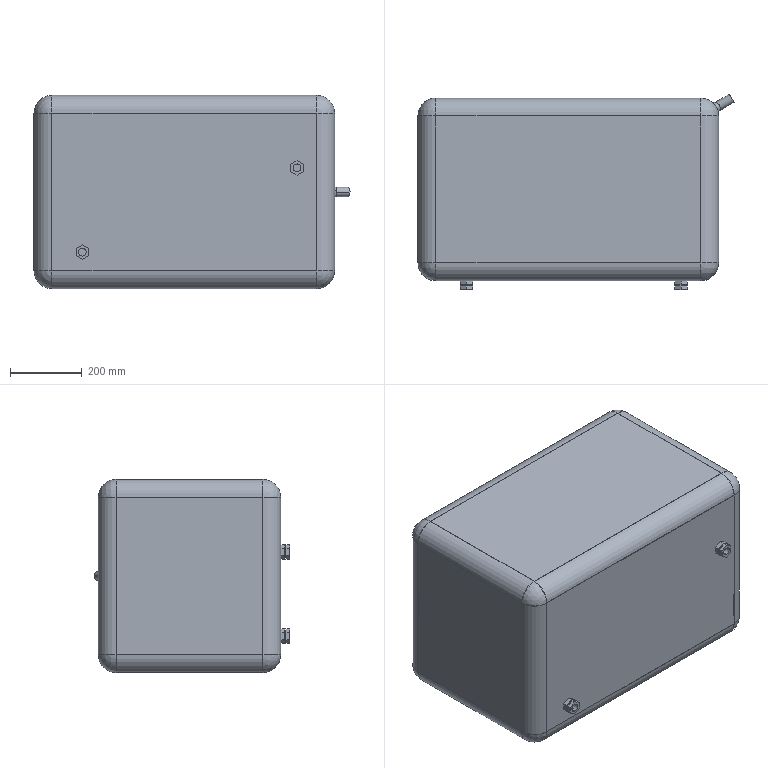Part | SolidWorks | features ICE 6, Fillet 2, Extrusion 1, Shell 1 | 1 solid | 97 faces | box 883.103 x 546.258 x 540 mm | volume 6439687 mm3 | plane 43 | cylinder 36 | sphere 16 | spline 2 | commonest cylinder face diameters 94 x12 100 x12 22 x4 30 x4 20 x2 26 x2